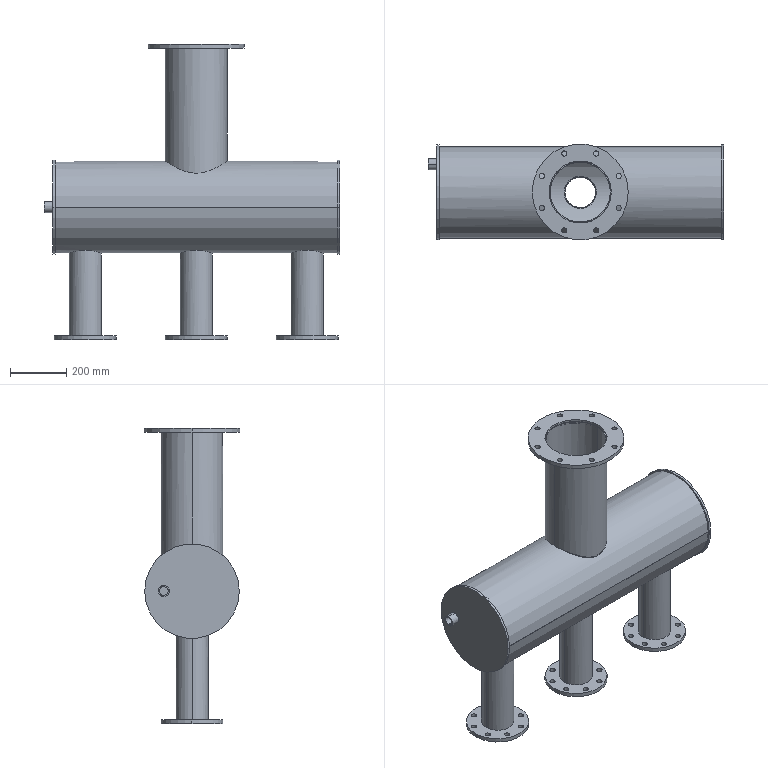Part | SolidWorks | features ICE 8, 3DProfileFeature 4, Extrusion 1, MoveCopyBody 1, Stock 1, Sweep 1, WeldmentFeature 1 | 12 solids | 142 faces | box 1046 x 340 x 1046 mm | volume 7874309 mm3 | cylinder 114 | plane 20 | spline 8 | commonest cylinder face diameters 18 x64 220 x8 108.3 x6 114.3 x6 115 x6 325 x6